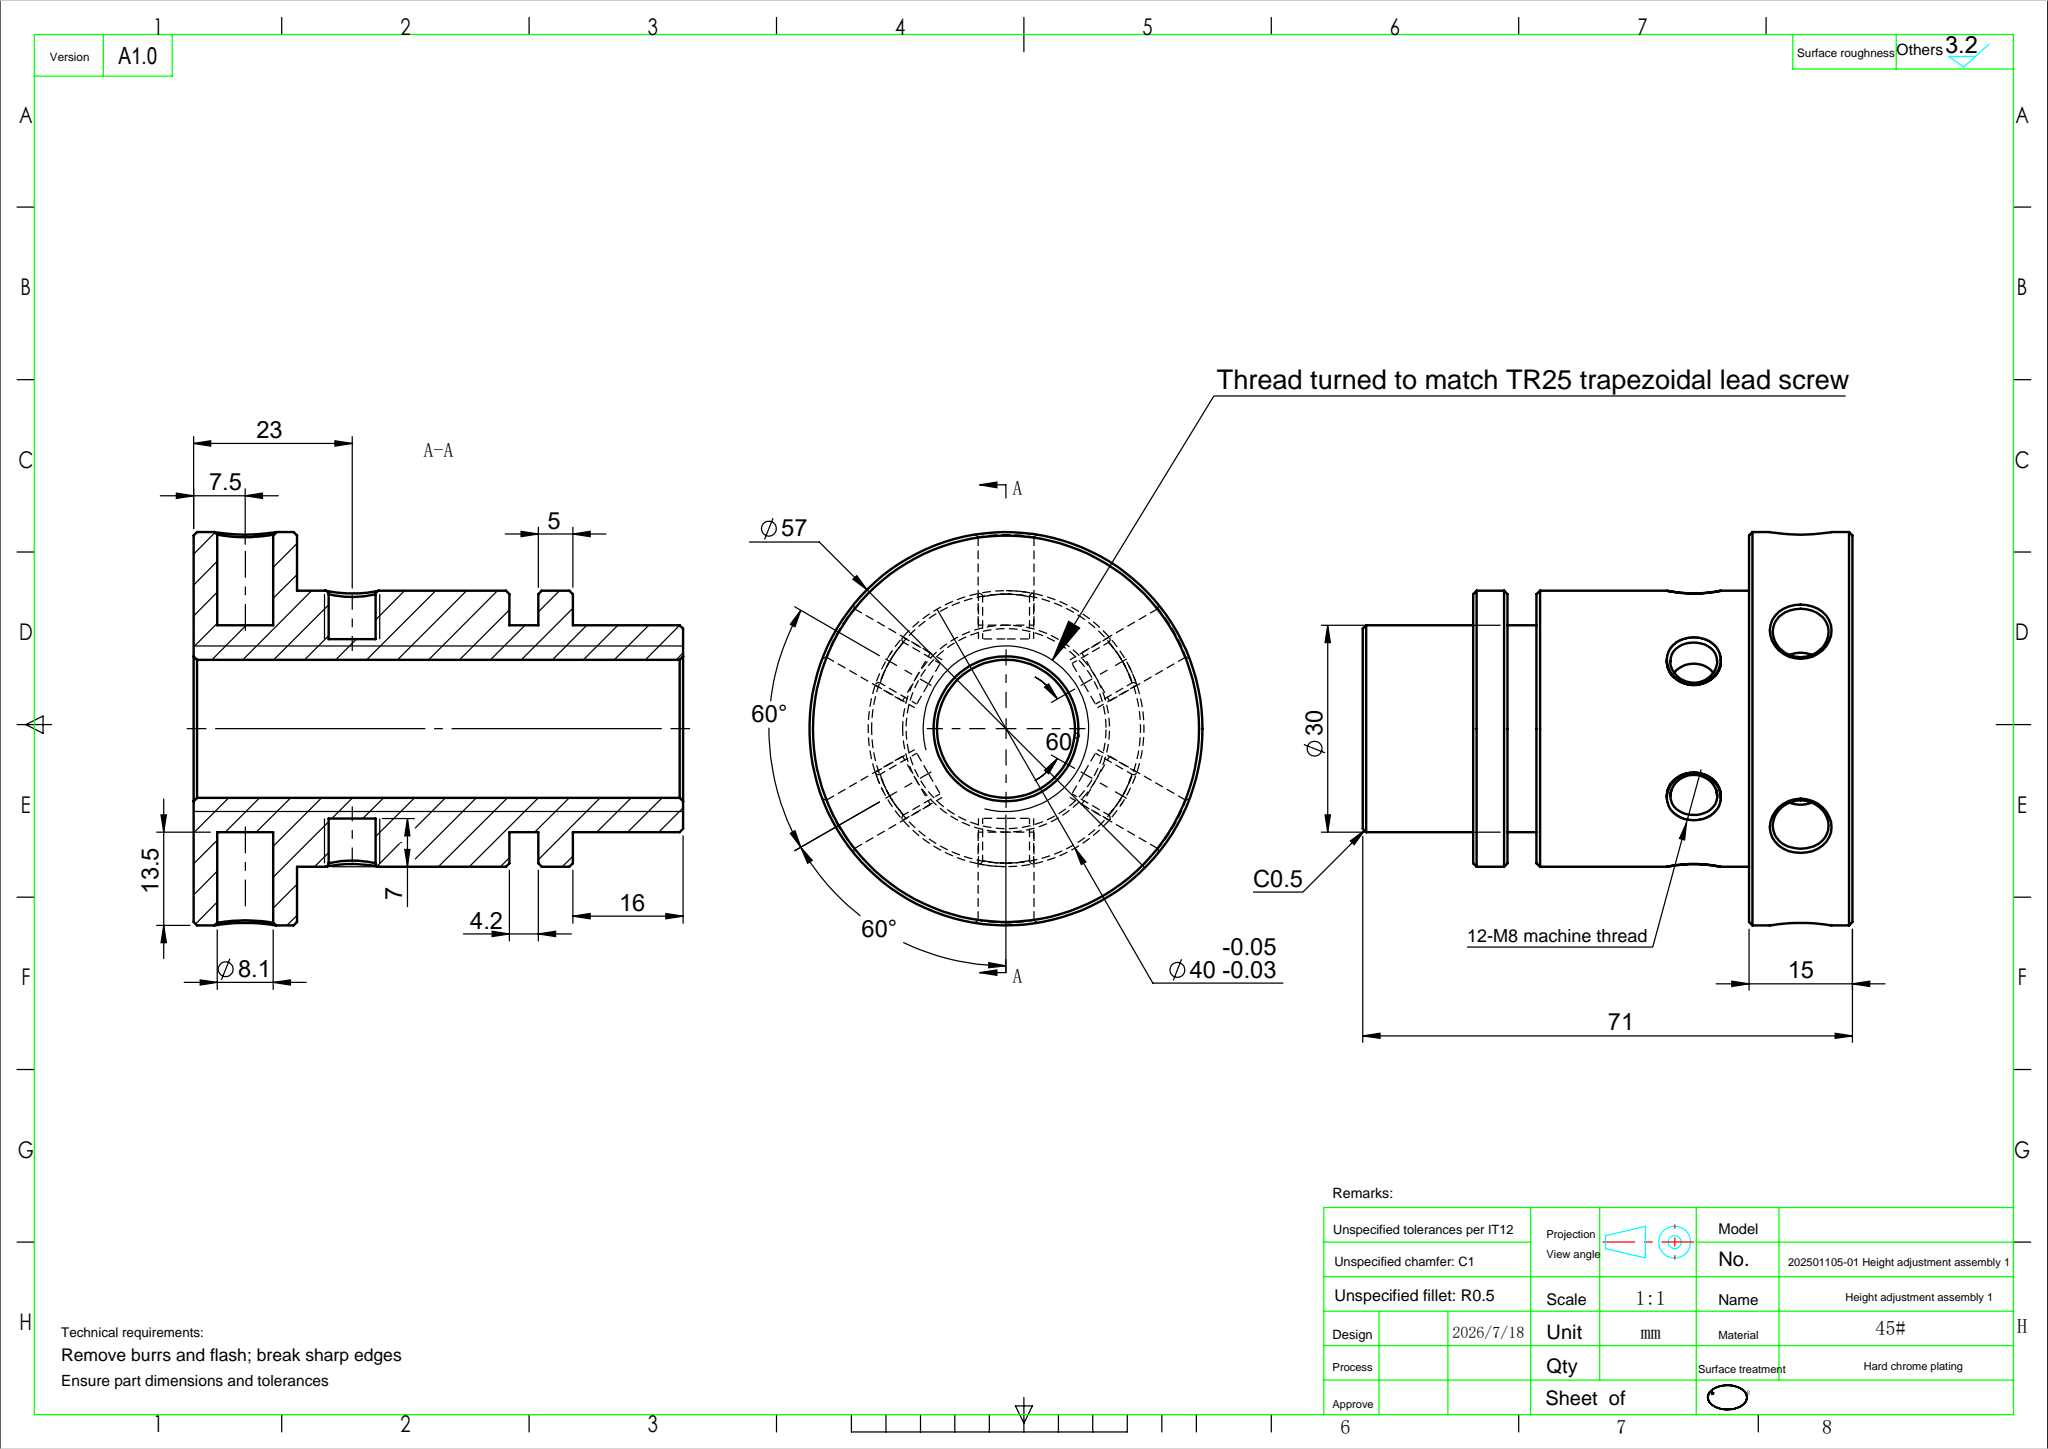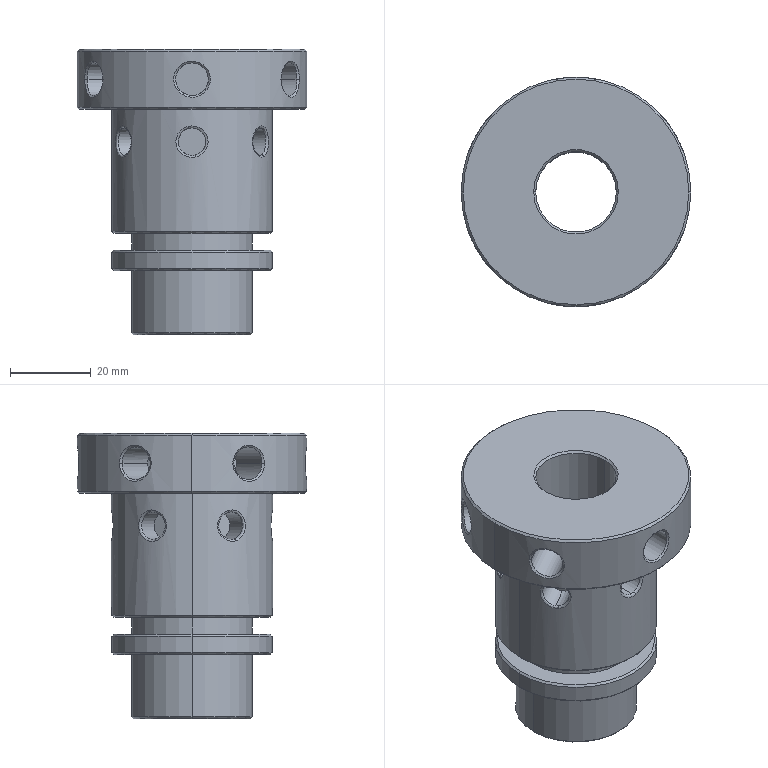Part | SolidWorks | features Chamfer 5, ICE 5, CirPattern 2, Extrusion 1, Fillet 1, MoveFace 1 | 1 solid | 94 faces | box 57 x 57 x 71 mm | volume 69434 mm3 | cylinder 36 | spline 24 | plane 18 | cone 16 | commonest cylinder face diameters 6.8 x12 8.1 x12 30 x4 40 x4 20 x2 57 x2